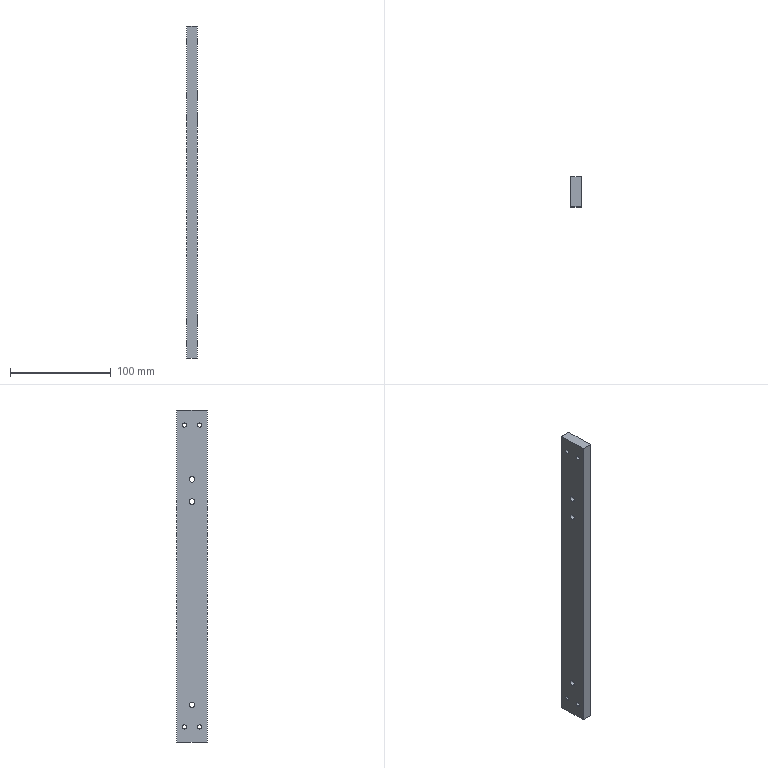Part | STEP file | 06-38 Heat-shrink tube support crossbar | 1 solid | 29 faces | box 10 x 30 x 330 mm | volume 96911 mm3 | cylinder 20 | plane 9 | commonest cylinder face diameters 4.2 x8 5.5 x6 10 x6